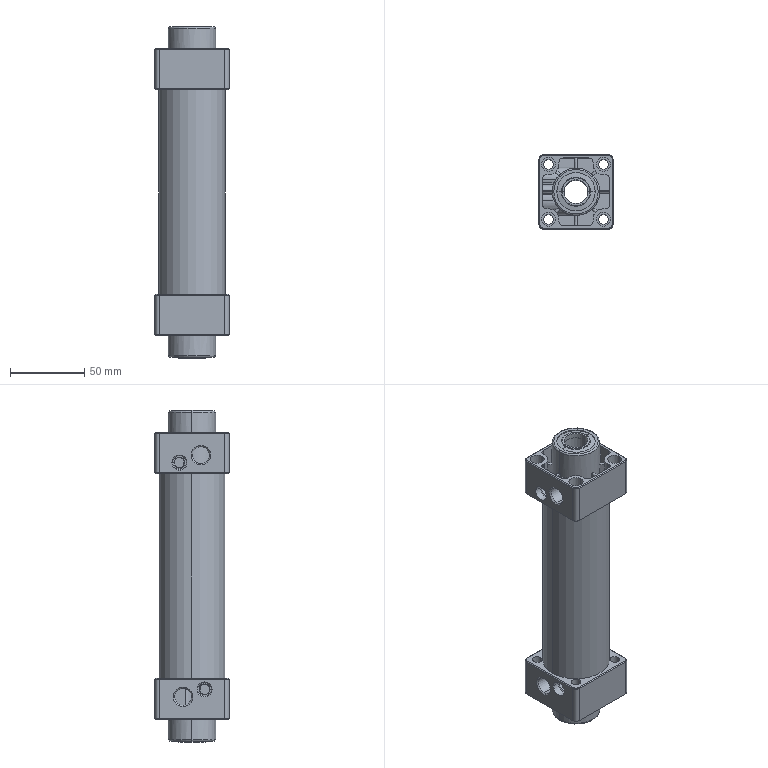Part | SolidWorks | features BaseBody 1 | 1 solid | 322 faces | box 50 x 50 x 224 mm | volume 150469 mm3 | cylinder 155 | plane 123 | cone 32 | torus 12 | commonest cylinder face diameters 6 x24 2 x20 6.5 x16 9.5 x16 16 x10 14 x8